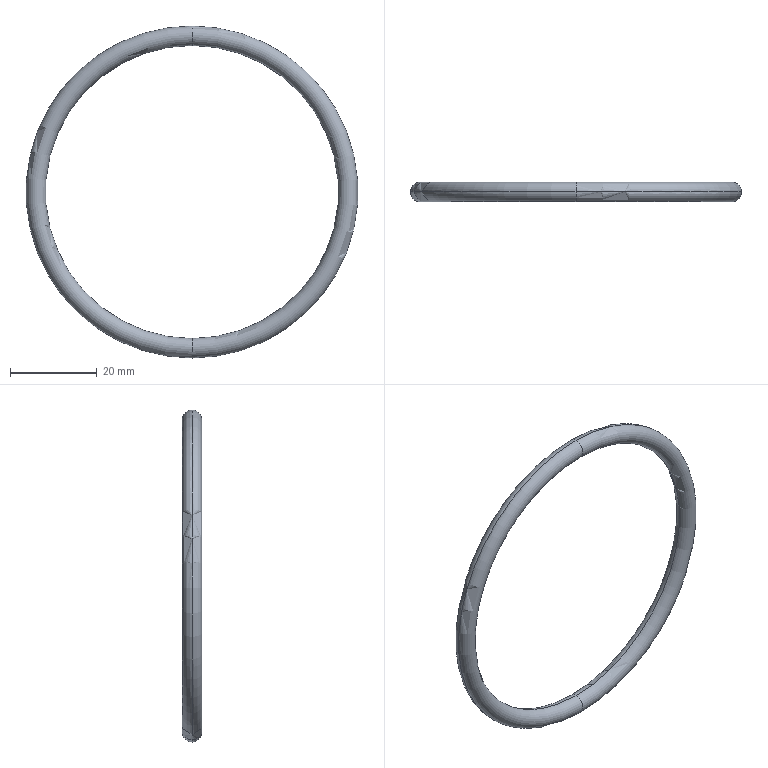Part | SolidWorks | features Revolution 1 | 1 solid | 4 faces | box 76.75 x 4.5 x 76.75 mm | volume 3610 mm3 | torus 4
STEP:
#1=CARTESIAN_POINT('',(0.,0.,38.375));
#2=VERTEX_POINT('',#1);
#3=CARTESIAN_POINT('',(0.,0.,33.875));
#4=VERTEX_POINT('',#3);
#5=CARTESIAN_POINT('',(0.,0.,36.125));
#6=DIRECTION('',(1.,0.,0.));
#7=DIRECTION('',(0.,0.,-1.));
#8=AXIS2_PLACEMENT_3D('',#5,#6,#7);
#9=CIRCLE('',#8,2.25);
#10=EDGE_CURVE('',#2,#4,#9,.T.);
#11=ORIENTED_EDGE('',*,*,#10,.F.);
#12=CARTESIAN_POINT('',(0.,0.,-38.375));
#13=VERTEX_POINT('',#12);
#14=CARTESIAN_POINT('',(0.,0.,0.));
#15=DIRECTION('',(0.,-1.,0.));
#16=DIRECTION('',(0.,0.,-1.));
#17=AXIS2_PLACEMENT_3D('',#14,#15,#16);
#18=CIRCLE('',#17,38.375);
#19=EDGE_CURVE('',#2,#13,#18,.T.);
#20=ORIENTED_EDGE('',*,*,#19,.T.);
#21=CARTESIAN_POINT('',(0.,0.,-33.875));
#22=VERTEX_POINT('',#21);
#23=CARTESIAN_POINT('',(0.,0.,-36.125));
#24=DIRECTION('',(-1.,0.,0.));
#25=DIRECTION('',(0.,0.,1.));
#26=AXIS2_PLACEMENT_3D('',#23,#24,#25);
#27=CIRCLE('',#26,2.25);
#28=EDGE_CURVE('',#13,#22,#27,.T.);
#29=ORIENTED_EDGE('',*,*,#28,.T.);
#30=CARTESIAN_POINT('',(0.,0.,0.));
#31=DIRECTION('',(0.,-1.,0.));
#32=DIRECTION('',(0.,0.,-1.));
#33=AXIS2_PLACEMENT_3D('',#30,#31,#32);
#34=CIRCLE('',#33,33.875);
#35=EDGE_CURVE('',#4,#22,#34,.T.);
#36=ORIENTED_EDGE('',*,*,#35,.F.);
#37=EDGE_LOOP('',(#11,#20,#29,#36));
#38=FACE_OUTER_BOUND('',#37,.T.);
#39=CARTESIAN_POINT('',(0.,0.,0.));
#40=DIRECTION('',(0.,-1.,0.));
#41=DIRECTION('',(0.,0.,-1.));
#42=AXIS2_PLACEMENT_3D('',#39,#40,#41);
#43=TOROIDAL_SURFACE('',#42,36.125,2.25);
#44=ADVANCED_FACE('',(#38),#43,.T.);
#45=ORIENTED_EDGE('',*,*,#28,.F.);
#46=CARTESIAN_POINT('',(0.,0.,0.));
#47=DIRECTION('',(0.,-1.,0.));
#48=DIRECTION('',(0.,0.,-1.));
#49=AXIS2_PLACEMENT_3D('',#46,#47,#48);
#50=CIRCLE('',#49,38.375);
#51=EDGE_CURVE('',#13,#2,#50,.T.);
#52=ORIENTED_EDGE('',*,*,#51,.T.);
#53=ORIENTED_EDGE('',*,*,#10,.T.);
#54=CARTESIAN_POINT('',(0.,0.,0.));
#55=DIRECTION('',(0.,-1.,0.));
#56=DIRECTION('',(0.,0.,-1.));
#57=AXIS2_PLACEMENT_3D('',#54,#55,#56);
#58=CIRCLE('',#57,33.875);
#59=EDGE_CURVE('',#22,#4,#58,.T.);
#60=ORIENTED_EDGE('',*,*,#59,.F.);
#61=EDGE_LOOP('',(#45,#52,#53,#60));
#62=FACE_OUTER_BOUND('',#61,.T.);
#63=CARTESIAN_POINT('',(0.,0.,0.));
#64=DIRECTION('',(0.,-1.,0.));
#65=DIRECTION('',(0.,0.,-1.));
#66=AXIS2_PLACEMENT_3D('',#63,#64,#65);
#67=TOROIDAL_SURFACE('',#66,36.125,2.25);
#68=ADVANCED_FACE('',(#62),#67,.T.);
#69=ORIENTED_EDGE('',*,*,#51,.F.);
#70=CARTESIAN_POINT('',(0.,0.,-36.125));
#71=DIRECTION('',(-1.,0.,0.));
#72=DIRECTION('',(0.,0.,1.));
#73=AXIS2_PLACEMENT_3D('',#70,#71,#72);
#74=CIRCLE('',#73,2.25);
#75=EDGE_CURVE('',#22,#13,#74,.T.);
#76=ORIENTED_EDGE('',*,*,#75,.F.);
#77=ORIENTED_EDGE('',*,*,#59,.T.);
#78=CARTESIAN_POINT('',(0.,0.,36.125));
#79=DIRECTION('',(1.,0.,0.));
#80=DIRECTION('',(0.,0.,-1.));
#81=AXIS2_PLACEMENT_3D('',#78,#79,#80);
#82=CIRCLE('',#81,2.25);
#83=EDGE_CURVE('',#4,#2,#82,.T.);
#84=ORIENTED_EDGE('',*,*,#83,.T.);
#85=EDGE_LOOP('',(#69,#76,#77,#84));
#86=FACE_OUTER_BOUND('',#85,.T.);
#87=CARTESIAN_POINT('',(0.,0.,0.));
#88=DIRECTION('',(0.,-1.,0.));
#89=DIRECTION('',(0.,0.,-1.));
#90=AXIS2_PLACEMENT_3D('',#87,#88,#89);
#91=TOROIDAL_SURFACE('',#90,36.125,2.25);
#92=ADVANCED_FACE('',(#86),#91,.T.);
#93=ORIENTED_EDGE('',*,*,#19,.F.);
#94=ORIENTED_EDGE('',*,*,#83,.F.);
#95=ORIENTED_EDGE('',*,*,#35,.T.);
#96=ORIENTED_EDGE('',*,*,#75,.T.);
#97=EDGE_LOOP('',(#93,#94,#95,#96));
#98=FACE_OUTER_BOUND('',#97,.T.);
#99=CARTESIAN_POINT('',(0.,0.,0.));
#100=DIRECTION('',(0.,-1.,0.));
#101=DIRECTION('',(0.,0.,-1.));
#102=AXIS2_PLACEMENT_3D('',#99,#100,#101);
#103=TOROIDAL_SURFACE('',#102,36.125,2.25);
#104=ADVANCED_FACE('',(#98),#103,.T.);
#105=CLOSED_SHELL('',(#44,#68,#92,#104));
#106=MANIFOLD_SOLID_BREP('',#105);
#107=CARTESIAN_POINT('',(0.,0.,0.));
#108=DIRECTION('',(0.,0.,1.));
#109=DIRECTION('',(1.,0.,0.));
#110=AXIS2_PLACEMENT_3D('',#107,#108,#109);
#111=(LENGTH_UNIT()NAMED_UNIT(*)SI_UNIT(.MILLI.,.METRE.));
#112=UNCERTAINTY_MEASURE_WITH_UNIT(LENGTH_MEASURE(0.00001),#111,'','');
#113=(NAMED_UNIT(*)PLANE_ANGLE_UNIT()SI_UNIT($,.RADIAN.));
#114=(NAMED_UNIT(*)SI_UNIT($,.STERADIAN.)SOLID_ANGLE_UNIT());
#115=(GEOMETRIC_REPRESENTATION_CONTEXT(3)GLOBAL_UNCERTAINTY_ASSIGNED_CONTEXT((#112))GLOBAL_UNIT_ASSIGNED_CONTEXT((#111,#113,#114))REPRESENTATION_CONTEXT('',''));
#116=ADVANCED_BREP_SHAPE_REPRESENTATION('',(#106,#110),#115);